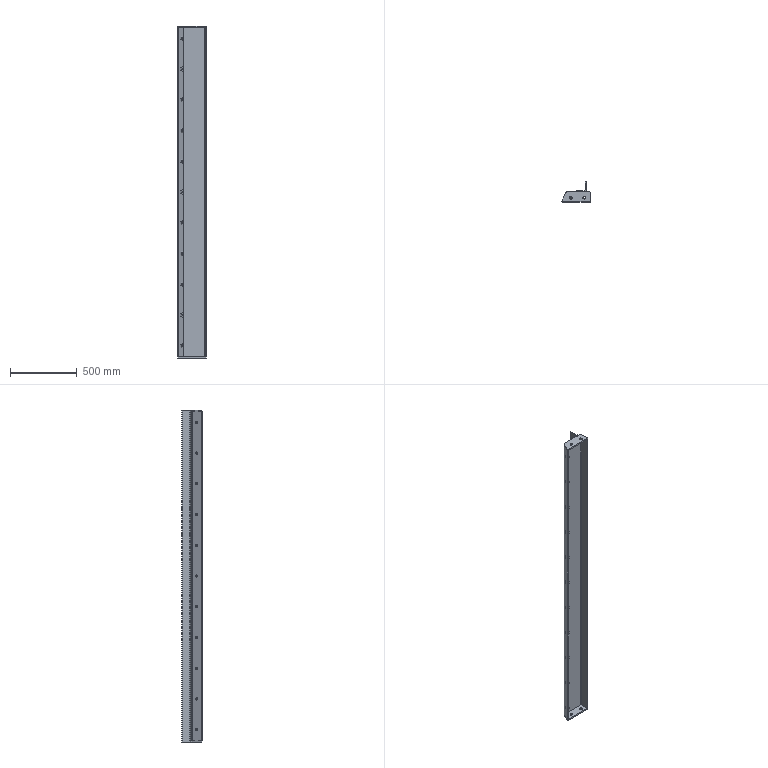Part | STEP file | Connecting beam 1_Default<As machined> | 15 solids | 183 faces | box 214 x 150.815 x 2484 mm | volume 9468856 mm3 | plane 120 | cylinder 63 | commonest cylinder face diameters 18 x23 14 x22 21 x8 20 x6 4 x2 5.333 x2